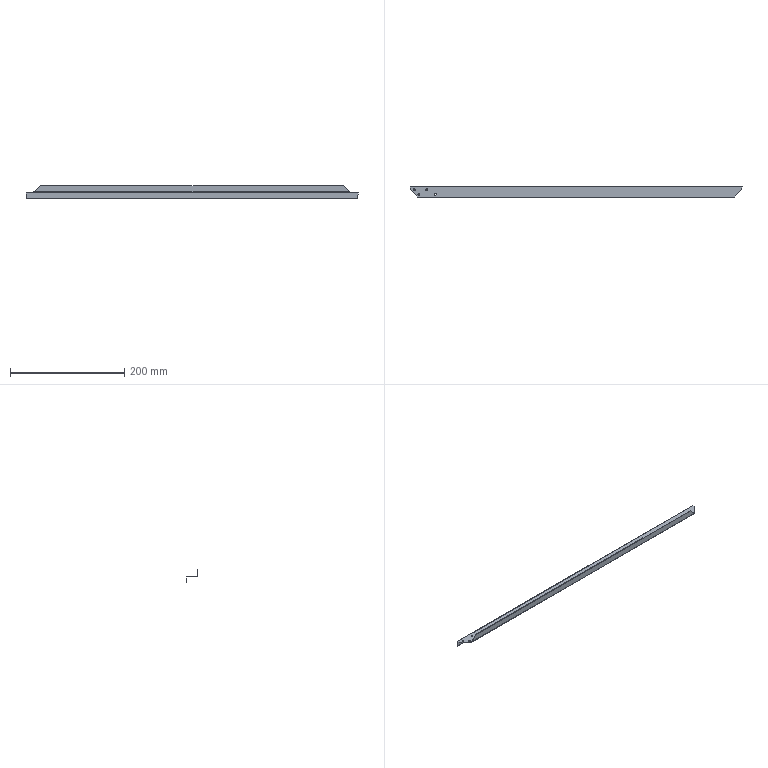Part | SolidWorks | features BaseBody 1 | 1 solid | 28 faces | box 580 x 20.861 x 22.562 mm | volume 11752 mm3 | plane 14 | cylinder 12 | spline 2 | commonest cylinder face diameters 3.2 x8 2 x2 3 x2
STEP:
#1=CARTESIAN_POINT('',(-272.991,-3.763,-0.5));
#2=VERTEX_POINT('',#1);
#3=CARTESIAN_POINT('',(-276.191,-3.763,-0.5));
#4=VERTEX_POINT('',#3);
#5=CARTESIAN_POINT('',(-274.591,-3.763,-0.5));
#6=DIRECTION('',(0.,0.,-1.));
#7=DIRECTION('',(1.,0.,0.));
#8=AXIS2_PLACEMENT_3D('',#5,#6,#7);
#9=CIRCLE('',#8,1.6);
#10=EDGE_CURVE('',#2,#4,#9,.T.);
#11=ORIENTED_EDGE('',*,*,#10,.T.);
#12=CARTESIAN_POINT('',(-276.191,-3.763,0.));
#13=VERTEX_POINT('',#12);
#14=CARTESIAN_POINT('',(-276.191,-3.763,-0.5));
#15=DIRECTION('',(0.,0.,1.));
#16=VECTOR('',#15,1000.);
#17=LINE('',#14,#16);
#18=EDGE_CURVE('',#4,#13,#17,.T.);
#19=ORIENTED_EDGE('',*,*,#18,.T.);
#20=CARTESIAN_POINT('',(-272.991,-3.763,0.));
#21=VERTEX_POINT('',#20);
#22=CARTESIAN_POINT('',(-274.591,-3.763,0.));
#23=DIRECTION('',(0.,0.,1.));
#24=DIRECTION('',(1.,0.,0.));
#25=AXIS2_PLACEMENT_3D('',#22,#23,#24);
#26=CIRCLE('',#25,1.6);
#27=EDGE_CURVE('',#13,#21,#26,.T.);
#28=ORIENTED_EDGE('',*,*,#27,.T.);
#29=CARTESIAN_POINT('',(-272.991,-3.763,-0.5));
#30=DIRECTION('',(0.,0.,1.));
#31=VECTOR('',#30,1000.);
#32=LINE('',#29,#31);
#33=EDGE_CURVE('',#2,#21,#32,.T.);
#34=ORIENTED_EDGE('',*,*,#33,.F.);
#35=EDGE_LOOP('',(#11,#19,#28,#34));
#36=FACE_OUTER_BOUND('',#35,.T.);
#37=CARTESIAN_POINT('',(-274.591,-3.763,-0.5));
#38=DIRECTION('',(0.,0.,1.));
#39=DIRECTION('',(1.,0.,0.));
#40=AXIS2_PLACEMENT_3D('',#37,#38,#39);
#41=CYLINDRICAL_SURFACE('',#40,1.6);
#42=ADVANCED_FACE('',(#36),#41,.F.);
#43=CARTESIAN_POINT('',(-284.191,4.237,-0.5));
#44=VERTEX_POINT('',#43);
#45=CARTESIAN_POINT('',(-280.991,4.237,-0.5));
#46=VERTEX_POINT('',#45);
#47=CARTESIAN_POINT('',(-282.591,4.237,-0.5));
#48=DIRECTION('',(0.,0.,1.));
#49=DIRECTION('',(1.,0.,0.));
#50=AXIS2_PLACEMENT_3D('',#47,#48,#49);
#51=CIRCLE('',#50,1.6);
#52=EDGE_CURVE('',#44,#46,#51,.T.);
#53=ORIENTED_EDGE('',*,*,#52,.F.);
#54=CARTESIAN_POINT('',(-284.191,4.237,0.));
#55=VERTEX_POINT('',#54);
#56=CARTESIAN_POINT('',(-284.191,4.237,-0.5));
#57=DIRECTION('',(0.,0.,1.));
#58=VECTOR('',#57,1000.);
#59=LINE('',#56,#58);
#60=EDGE_CURVE('',#44,#55,#59,.T.);
#61=ORIENTED_EDGE('',*,*,#60,.T.);
#62=CARTESIAN_POINT('',(-280.991,4.237,0.));
#63=VERTEX_POINT('',#62);
#64=CARTESIAN_POINT('',(-282.591,4.237,0.));
#65=DIRECTION('',(0.,0.,1.));
#66=DIRECTION('',(1.,0.,0.));
#67=AXIS2_PLACEMENT_3D('',#64,#65,#66);
#68=CIRCLE('',#67,1.6);
#69=EDGE_CURVE('',#55,#63,#68,.T.);
#70=ORIENTED_EDGE('',*,*,#69,.T.);
#71=CARTESIAN_POINT('',(-280.991,4.237,-0.5));
#72=DIRECTION('',(0.,0.,1.));
#73=VECTOR('',#72,1000.);
#74=LINE('',#71,#73);
#75=EDGE_CURVE('',#46,#63,#74,.T.);
#76=ORIENTED_EDGE('',*,*,#75,.F.);
#77=EDGE_LOOP('',(#53,#61,#70,#76));
#78=FACE_OUTER_BOUND('',#77,.T.);
#79=CARTESIAN_POINT('',(-282.591,4.237,-0.5));
#80=DIRECTION('',(0.,0.,1.));
#81=DIRECTION('',(1.,0.,0.));
#82=AXIS2_PLACEMENT_3D('',#79,#80,#81);
#83=CYLINDRICAL_SURFACE('',#82,1.6);
#84=ADVANCED_FACE('',(#78),#83,.F.);
#85=CARTESIAN_POINT('',(-262.191,4.237,-0.5));
#86=VERTEX_POINT('',#85);
#87=CARTESIAN_POINT('',(-258.991,4.237,-0.5));
#88=VERTEX_POINT('',#87);
#89=CARTESIAN_POINT('',(-260.591,4.237,-0.5));
#90=DIRECTION('',(0.,0.,1.));
#91=DIRECTION('',(1.,0.,0.));
#92=AXIS2_PLACEMENT_3D('',#89,#90,#91);
#93=CIRCLE('',#92,1.6);
#94=EDGE_CURVE('',#86,#88,#93,.T.);
#95=ORIENTED_EDGE('',*,*,#94,.F.);
#96=CARTESIAN_POINT('',(-262.191,4.237,0.));
#97=VERTEX_POINT('',#96);
#98=CARTESIAN_POINT('',(-262.191,4.237,-0.5));
#99=DIRECTION('',(0.,0.,1.));
#100=VECTOR('',#99,1000.);
#101=LINE('',#98,#100);
#102=EDGE_CURVE('',#86,#97,#101,.T.);
#103=ORIENTED_EDGE('',*,*,#102,.T.);
#104=CARTESIAN_POINT('',(-258.991,4.237,0.));
#105=VERTEX_POINT('',#104);
#106=CARTESIAN_POINT('',(-260.591,4.237,0.));
#107=DIRECTION('',(0.,0.,1.));
#108=DIRECTION('',(1.,0.,0.));
#109=AXIS2_PLACEMENT_3D('',#106,#107,#108);
#110=CIRCLE('',#109,1.6);
#111=EDGE_CURVE('',#97,#105,#110,.T.);
#112=ORIENTED_EDGE('',*,*,#111,.T.);
#113=CARTESIAN_POINT('',(-258.991,4.237,-0.5));
#114=DIRECTION('',(0.,0.,1.));
#115=VECTOR('',#114,1000.);
#116=LINE('',#113,#115);
#117=EDGE_CURVE('',#88,#105,#116,.T.);
#118=ORIENTED_EDGE('',*,*,#117,.F.);
#119=EDGE_LOOP('',(#95,#103,#112,#118));
#120=FACE_OUTER_BOUND('',#119,.T.);
#121=CARTESIAN_POINT('',(-260.591,4.237,-0.5));
#122=DIRECTION('',(0.,0.,1.));
#123=DIRECTION('',(1.,0.,0.));
#124=AXIS2_PLACEMENT_3D('',#121,#122,#123);
#125=CYLINDRICAL_SURFACE('',#124,1.6);
#126=ADVANCED_FACE('',(#120),#125,.F.);
#127=CARTESIAN_POINT('',(-247.581,-3.763,-0.5));
#128=VERTEX_POINT('',#127);
#129=CARTESIAN_POINT('',(-244.381,-3.763,-0.5));
#130=VERTEX_POINT('',#129);
#131=CARTESIAN_POINT('',(-245.981,-3.763,-0.5));
#132=DIRECTION('',(0.,0.,1.));
#133=DIRECTION('',(1.,0.,0.));
#134=AXIS2_PLACEMENT_3D('',#131,#132,#133);
#135=CIRCLE('',#134,1.6);
#136=EDGE_CURVE('',#128,#130,#135,.T.);
#137=ORIENTED_EDGE('',*,*,#136,.F.);
#138=CARTESIAN_POINT('',(-247.581,-3.763,0.));
#139=VERTEX_POINT('',#138);
#140=CARTESIAN_POINT('',(-247.581,-3.763,-0.5));
#141=DIRECTION('',(0.,0.,1.));
#142=VECTOR('',#141,1000.);
#143=LINE('',#140,#142);
#144=EDGE_CURVE('',#128,#139,#143,.T.);
#145=ORIENTED_EDGE('',*,*,#144,.T.);
#146=CARTESIAN_POINT('',(-244.381,-3.763,0.));
#147=VERTEX_POINT('',#146);
#148=CARTESIAN_POINT('',(-245.981,-3.763,0.));
#149=DIRECTION('',(0.,0.,1.));
#150=DIRECTION('',(1.,0.,0.));
#151=AXIS2_PLACEMENT_3D('',#148,#149,#150);
#152=CIRCLE('',#151,1.6);
#153=EDGE_CURVE('',#139,#147,#152,.T.);
#154=ORIENTED_EDGE('',*,*,#153,.T.);
#155=CARTESIAN_POINT('',(-244.381,-3.763,-0.5));
#156=DIRECTION('',(0.,0.,1.));
#157=VECTOR('',#156,1000.);
#158=LINE('',#155,#157);
#159=EDGE_CURVE('',#130,#147,#158,.T.);
#160=ORIENTED_EDGE('',*,*,#159,.F.);
#161=EDGE_LOOP('',(#137,#145,#154,#160));
#162=FACE_OUTER_BOUND('',#161,.T.);
#163=CARTESIAN_POINT('',(-245.981,-3.763,-0.5));
#164=DIRECTION('',(0.,0.,1.));
#165=DIRECTION('',(1.,0.,0.));
#166=AXIS2_PLACEMENT_3D('',#163,#164,#165);
#167=CYLINDRICAL_SURFACE('',#166,1.6);
#168=ADVANCED_FACE('',(#162),#167,.F.);
#169=ORIENTED_EDGE('',*,*,#18,.F.);
#170=CARTESIAN_POINT('',(-274.591,-3.763,-0.5));
#171=DIRECTION('',(0.,0.,-1.));
#172=DIRECTION('',(1.,0.,0.));
#173=AXIS2_PLACEMENT_3D('',#170,#171,#172);
#174=CIRCLE('',#173,1.6);
#175=EDGE_CURVE('',#4,#2,#174,.T.);
#176=ORIENTED_EDGE('',*,*,#175,.T.);
#177=ORIENTED_EDGE('',*,*,#33,.T.);
#178=CARTESIAN_POINT('',(-274.591,-3.763,0.));
#179=DIRECTION('',(0.,0.,1.));
#180=DIRECTION('',(1.,0.,0.));
#181=AXIS2_PLACEMENT_3D('',#178,#179,#180);
#182=CIRCLE('',#181,1.6);
#183=EDGE_CURVE('',#21,#13,#182,.T.);
#184=ORIENTED_EDGE('',*,*,#183,.T.);
#185=EDGE_LOOP('',(#169,#176,#177,#184));
#186=FACE_OUTER_BOUND('',#185,.T.);
#187=CARTESIAN_POINT('',(-274.591,-3.763,-0.5));
#188=DIRECTION('',(0.,0.,1.));
#189=DIRECTION('',(1.,0.,0.));
#190=AXIS2_PLACEMENT_3D('',#187,#188,#189);
#191=CYLINDRICAL_SURFACE('',#190,1.6);
#192=ADVANCED_FACE('',(#186),#191,.F.);
#193=CARTESIAN_POINT('',(-282.591,4.237,0.));
#194=DIRECTION('',(0.,0.,1.));
#195=DIRECTION('',(1.,0.,0.));
#196=AXIS2_PLACEMENT_3D('',#193,#194,#195);
#197=CIRCLE('',#196,1.6);
#198=EDGE_CURVE('',#63,#55,#197,.T.);
#199=ORIENTED_EDGE('',*,*,#198,.F.);
#200=ORIENTED_EDGE('',*,*,#69,.F.);
#201=EDGE_LOOP('',(#199,#200));
#202=FACE_BOUND('',#201,.T.);
#203=CARTESIAN_POINT('',(-260.591,4.237,0.));
#204=DIRECTION('',(0.,0.,1.));
#205=DIRECTION('',(1.,0.,0.));
#206=AXIS2_PLACEMENT_3D('',#203,#204,#205);
#207=CIRCLE('',#206,1.6);
#208=EDGE_CURVE('',#105,#97,#207,.T.);
#209=ORIENTED_EDGE('',*,*,#208,.F.);
#210=ORIENTED_EDGE('',*,*,#111,.F.);
#211=EDGE_LOOP('',(#209,#210));
#212=FACE_BOUND('',#211,.T.);
#213=CARTESIAN_POINT('',(-245.981,-3.763,0.));
#214=DIRECTION('',(0.,0.,1.));
#215=DIRECTION('',(1.,0.,0.));
#216=AXIS2_PLACEMENT_3D('',#213,#214,#215);
#217=CIRCLE('',#216,1.6);
#218=EDGE_CURVE('',#147,#139,#217,.T.);
#219=ORIENTED_EDGE('',*,*,#218,.F.);
#220=ORIENTED_EDGE('',*,*,#153,.F.);
#221=EDGE_LOOP('',(#219,#220));
#222=FACE_BOUND('',#221,.T.);
#223=ORIENTED_EDGE('',*,*,#183,.F.);
#224=ORIENTED_EDGE('',*,*,#27,.F.);
#225=EDGE_LOOP('',(#223,#224));
#226=FACE_BOUND('',#225,.T.);
#227=CARTESIAN_POINT('',(276.986,-8.364,0.));
#228=VERTEX_POINT('',#227);
#229=CARTESIAN_POINT('',(-276.986,-8.364,0.));
#230=VERTEX_POINT('',#229);
#231=CARTESIAN_POINT('',(0.,-8.364,0.));
#232=DIRECTION('',(-1.,0.,0.));
#233=VECTOR('',#232,1000.);
#234=LINE('',#231,#233);
#235=EDGE_CURVE('',#228,#230,#234,.T.);
#236=ORIENTED_EDGE('',*,*,#235,.F.);
#237=CARTESIAN_POINT('',(290.,4.65,0.));
#238=VERTEX_POINT('',#237);
#239=CARTESIAN_POINT('',(276.986,-8.364,0.));
#240=DIRECTION('',(-0.7071,-0.7071,0.));
#241=VECTOR('',#240,1000.);
#242=LINE('',#239,#241);
#243=EDGE_CURVE('',#238,#228,#242,.T.);
#244=ORIENTED_EDGE('',*,*,#243,.F.);
#245=CARTESIAN_POINT('',(290.,9.35,0.));
#246=VERTEX_POINT('',#245);
#247=CARTESIAN_POINT('',(290.,0.4931,0.));
#248=DIRECTION('',(0.,-1.,0.));
#249=VECTOR('',#248,1000.);
#250=LINE('',#247,#249);
#251=EDGE_CURVE('',#246,#238,#250,.T.);
#252=ORIENTED_EDGE('',*,*,#251,.F.);
#253=CARTESIAN_POINT('',(-290.,9.35,0.));
#254=VERTEX_POINT('',#253);
#255=CARTESIAN_POINT('',(0.,9.35,0.));
#256=DIRECTION('',(1.,0.,0.));
#257=VECTOR('',#256,1000.);
#258=LINE('',#255,#257);
#259=EDGE_CURVE('',#254,#246,#258,.T.);
#260=ORIENTED_EDGE('',*,*,#259,.F.);
#261=CARTESIAN_POINT('',(-290.,4.65,0.));
#262=VERTEX_POINT('',#261);
#263=CARTESIAN_POINT('',(-290.,0.4931,0.));
#264=DIRECTION('',(0.,1.,0.));
#265=VECTOR('',#264,1000.);
#266=LINE('',#263,#265);
#267=EDGE_CURVE('',#262,#254,#266,.T.);
#268=ORIENTED_EDGE('',*,*,#267,.F.);
#269=CARTESIAN_POINT('',(-290.,4.65,0.));
#270=DIRECTION('',(-0.7071,0.7071,0.));
#271=VECTOR('',#270,1000.);
#272=LINE('',#269,#271);
#273=EDGE_CURVE('',#230,#262,#272,.T.);
#274=ORIENTED_EDGE('',*,*,#273,.F.);
#275=EDGE_LOOP('',(#236,#244,#252,#260,#268,#274));
#276=FACE_OUTER_BOUND('',#275,.T.);
#277=CARTESIAN_POINT('',(290.,-8.364,0.));
#278=DIRECTION('',(0.,0.,-1.));
#279=DIRECTION('',(-1.,0.,0.));
#280=AXIS2_PLACEMENT_3D('',#277,#278,#279);
#281=PLANE('',#280);
#282=ADVANCED_FACE('',(#202,#212,#222,#226,#276),#281,.F.);
#283=CARTESIAN_POINT('',(-282.591,4.237,-0.5));
#284=DIRECTION('',(0.,0.,1.));
#285=DIRECTION('',(1.,0.,0.));
#286=AXIS2_PLACEMENT_3D('',#283,#284,#285);
#287=CIRCLE('',#286,1.6);
#288=EDGE_CURVE('',#46,#44,#287,.T.);
#289=ORIENTED_EDGE('',*,*,#288,.T.);
#290=ORIENTED_EDGE('',*,*,#52,.T.);
#291=EDGE_LOOP('',(#289,#290));
#292=FACE_BOUND('',#291,.T.);
#293=CARTESIAN_POINT('',(-260.591,4.237,-0.5));
#294=DIRECTION('',(0.,0.,1.));
#295=DIRECTION('',(1.,0.,0.));
#296=AXIS2_PLACEMENT_3D('',#293,#294,#295);
#297=CIRCLE('',#296,1.6);
#298=EDGE_CURVE('',#88,#86,#297,.T.);
#299=ORIENTED_EDGE('',*,*,#298,.T.);
#300=ORIENTED_EDGE('',*,*,#94,.T.);
#301=EDGE_LOOP('',(#299,#300));
#302=FACE_BOUND('',#301,.T.);
#303=CARTESIAN_POINT('',(-245.981,-3.763,-0.5));
#304=DIRECTION('',(0.,0.,1.));
#305=DIRECTION('',(1.,0.,0.));
#306=AXIS2_PLACEMENT_3D('',#303,#304,#305);
#307=CIRCLE('',#306,1.6);
#308=EDGE_CURVE('',#130,#128,#307,.T.);
#309=ORIENTED_EDGE('',*,*,#308,.T.);
#310=ORIENTED_EDGE('',*,*,#136,.T.);
#311=EDGE_LOOP('',(#309,#310));
#312=FACE_BOUND('',#311,.T.);
#313=ORIENTED_EDGE('',*,*,#10,.F.);
#314=ORIENTED_EDGE('',*,*,#175,.F.);
#315=EDGE_LOOP('',(#313,#314));
#316=FACE_BOUND('',#315,.T.);
#317=CARTESIAN_POINT('',(290.,9.35,-0.5));
#318=VERTEX_POINT('',#317);
#319=CARTESIAN_POINT('',(290.,4.65,-0.5));
#320=VERTEX_POINT('',#319);
#321=CARTESIAN_POINT('',(290.,0.4931,-0.5));
#322=DIRECTION('',(0.,-1.,0.));
#323=VECTOR('',#322,1000.);
#324=LINE('',#321,#323);
#325=EDGE_CURVE('',#318,#320,#324,.T.);
#326=ORIENTED_EDGE('',*,*,#325,.T.);
#327=CARTESIAN_POINT('',(276.986,-8.364,-0.5));
#328=VERTEX_POINT('',#327);
#329=CARTESIAN_POINT('',(290.,4.65,-0.5));
#330=DIRECTION('',(-0.7071,-0.7071,0.));
#331=VECTOR('',#330,1000.);
#332=LINE('',#329,#331);
#333=EDGE_CURVE('',#320,#328,#332,.T.);
#334=ORIENTED_EDGE('',*,*,#333,.T.);
#335=CARTESIAN_POINT('',(-276.986,-8.364,-0.5));
#336=VERTEX_POINT('',#335);
#337=CARTESIAN_POINT('',(0.,-8.364,-0.5));
#338=DIRECTION('',(-1.,0.,0.));
#339=VECTOR('',#338,1000.);
#340=LINE('',#337,#339);
#341=EDGE_CURVE('',#328,#336,#340,.T.);
#342=ORIENTED_EDGE('',*,*,#341,.T.);
#343=CARTESIAN_POINT('',(-290.,4.65,-0.5));
#344=VERTEX_POINT('',#343);
#345=CARTESIAN_POINT('',(-276.986,-8.364,-0.5));
#346=DIRECTION('',(-0.7071,0.7071,0.));
#347=VECTOR('',#346,1000.);
#348=LINE('',#345,#347);
#349=EDGE_CURVE('',#336,#344,#348,.T.);
#350=ORIENTED_EDGE('',*,*,#349,.T.);
#351=CARTESIAN_POINT('',(-290.,9.35,-0.5));
#352=VERTEX_POINT('',#351);
#353=CARTESIAN_POINT('',(-290.,0.4931,-0.5));
#354=DIRECTION('',(0.,1.,0.));
#355=VECTOR('',#354,1000.);
#356=LINE('',#353,#355);
#357=EDGE_CURVE('',#344,#352,#356,.T.);
#358=ORIENTED_EDGE('',*,*,#357,.T.);
#359=CARTESIAN_POINT('',(0.,9.35,-0.5));
#360=DIRECTION('',(1.,0.,0.));
#361=VECTOR('',#360,1000.);
#362=LINE('',#359,#361);
#363=EDGE_CURVE('',#352,#318,#362,.T.);
#364=ORIENTED_EDGE('',*,*,#363,.T.);
#365=EDGE_LOOP('',(#326,#334,#342,#350,#358,#364));
#366=FACE_OUTER_BOUND('',#365,.T.);
#367=CARTESIAN_POINT('',(290.,-8.364,-0.5));
#368=DIRECTION('',(0.,0.,-1.));
#369=DIRECTION('',(-1.,0.,0.));
#370=AXIS2_PLACEMENT_3D('',#367,#368,#369);
#371=PLANE('',#370);
#372=ADVANCED_FACE('',(#292,#302,#312,#316,#366),#371,.T.);
#373=ORIENTED_EDGE('',*,*,#60,.F.);
#374=ORIENTED_EDGE('',*,*,#288,.F.);
#375=ORIENTED_EDGE('',*,*,#75,.T.);
#376=ORIENTED_EDGE('',*,*,#198,.T.);
#377=EDGE_LOOP('',(#373,#374,#375,#376));
#378=FACE_OUTER_BOUND('',#377,.T.);
#379=CARTESIAN_POINT('',(-282.591,4.237,-0.5));
#380=DIRECTION('',(0.,0.,1.));
#381=DIRECTION('',(1.,0.,0.));
#382=AXIS2_PLACEMENT_3D('',#379,#380,#381);
#383=CYLINDRICAL_SURFACE('',#382,1.6);
#384=ADVANCED_FACE('',(#378),#383,.F.);
#385=ORIENTED_EDGE('',*,*,#102,.F.);
#386=ORIENTED_EDGE('',*,*,#298,.F.);
#387=ORIENTED_EDGE('',*,*,#117,.T.);
#388=ORIENTED_EDGE('',*,*,#208,.T.);
#389=EDGE_LOOP('',(#385,#386,#387,#388));
#390=FACE_OUTER_BOUND('',#389,.T.);
#391=CARTESIAN_POINT('',(-260.591,4.237,-0.5));
#392=DIRECTION('',(0.,0.,1.));
#393=DIRECTION('',(1.,0.,0.));
#394=AXIS2_PLACEMENT_3D('',#391,#392,#393);
#395=CYLINDRICAL_SURFACE('',#394,1.6);
#396=ADVANCED_FACE('',(#390),#395,.F.);
#397=ORIENTED_EDGE('',*,*,#144,.F.);
#398=ORIENTED_EDGE('',*,*,#308,.F.);
#399=ORIENTED_EDGE('',*,*,#159,.T.);
#400=ORIENTED_EDGE('',*,*,#218,.T.);
#401=EDGE_LOOP('',(#397,#398,#399,#400));
#402=FACE_OUTER_BOUND('',#401,.T.);
#403=CARTESIAN_POINT('',(-245.981,-3.763,-0.5));
#404=DIRECTION('',(0.,0.,1.));
#405=DIRECTION('',(1.,0.,0.));
#406=AXIS2_PLACEMENT_3D('',#403,#404,#405);
#407=CYLINDRICAL_SURFACE('',#406,1.6);
#408=ADVANCED_FACE('',(#402),#407,.F.);
#409=CARTESIAN_POINT('',(-290.,4.65,-0.25));
#410=DIRECTION('',(0.,0.,-1.));
#411=VECTOR('',#410,1000.);
#412=LINE('',#409,#411);
#413=EDGE_CURVE('',#262,#344,#412,.T.);
#414=ORIENTED_EDGE('',*,*,#413,.T.);
#415=ORIENTED_EDGE('',*,*,#349,.F.);
#416=CARTESIAN_POINT('',(-276.986,-8.364,-0.25));
#417=DIRECTION('',(0.,0.,-1.));
#418=VECTOR('',#417,1000.);
#419=LINE('',#416,#418);
#420=EDGE_CURVE('',#230,#336,#419,.T.);
#421=ORIENTED_EDGE('',*,*,#420,.F.);
#422=ORIENTED_EDGE('',*,*,#273,.T.);
#423=EDGE_LOOP('',(#414,#415,#421,#422));
#424=FACE_OUTER_BOUND('',#423,.T.);
#425=CARTESIAN_POINT('',(-290.,4.65,-0.5));
#426=DIRECTION('',(-0.7071,-0.7071,0.));
#427=DIRECTION('',(0.7071,-0.7071,0.));
#428=AXIS2_PLACEMENT_3D('',#425,#426,#427);
#429=PLANE('',#428);
#430=ADVANCED_FACE('',(#424),#429,.T.);
#431=CARTESIAN_POINT('',(-275.04,-9.364,0.986));
#432=VERTEX_POINT('',#431);
#433=CARTESIAN_POINT('',(275.04,-9.364,0.986));
#434=VERTEX_POINT('',#433);
#435=CARTESIAN_POINT('',(0.,-9.364,0.986));
#436=DIRECTION('',(1.,0.,0.));
#437=VECTOR('',#436,1000.);
#438=LINE('',#435,#437);
#439=EDGE_CURVE('',#432,#434,#438,.T.);
#440=ORIENTED_EDGE('',*,*,#439,.T.);
#441=CARTESIAN_POINT('',(275.04,-9.364,0.986));
#442=CARTESIAN_POINT('',(275.204,-9.362,0.8552));
#443=CARTESIAN_POINT('',(275.364,-9.335,0.7274));
#444=CARTESIAN_POINT('',(275.687,-9.233,0.4893));
#445=CARTESIAN_POINT('',(275.851,-9.158,0.3789));
#446=CARTESIAN_POINT('',(276.174,-8.974,0.1976));
#447=CARTESIAN_POINT('',(276.337,-8.864,0.1243));
#448=CARTESIAN_POINT('',(276.662,-8.623,0.02551));
#449=CARTESIAN_POINT('',(276.823,-8.495,0.000000001));
#450=CARTESIAN_POINT('',(276.986,-8.364,0.));
#451=B_SPLINE_CURVE_WITH_KNOTS('',3,(#441,#442,#443,#444,#445,#446,#447,#448,#449,#450),.UNSPECIFIED.,.F.,.F.,(4,2,2,2,4),(0.,0.0006197,0.001239,0.001859,0.002479),.UNSPECIFIED.);
#452=EDGE_CURVE('',#434,#228,#451,.T.);
#453=ORIENTED_EDGE('',*,*,#452,.T.);
#454=ORIENTED_EDGE('',*,*,#235,.T.);
#455=CARTESIAN_POINT('',(-276.986,-8.364,0.));
#456=CARTESIAN_POINT('',(-276.823,-8.495,0.000000002));
#457=CARTESIAN_POINT('',(-276.662,-8.623,0.02551));
#458=CARTESIAN_POINT('',(-276.339,-8.862,0.1235));
#459=CARTESIAN_POINT('',(-276.175,-8.974,0.1971));
#460=CARTESIAN_POINT('',(-275.852,-9.158,0.3783));
#461=CARTESIAN_POINT('',(-275.689,-9.233,0.4878));
#462=CARTESIAN_POINT('',(-275.364,-9.335,0.727));
#463=CARTESIAN_POINT('',(-275.204,-9.362,0.8552));
#464=CARTESIAN_POINT('',(-275.04,-9.364,0.986));
#465=B_SPLINE_CURVE_WITH_KNOTS('',3,(#455,#456,#457,#458,#459,#460,#461,#462,#463,#464),.UNSPECIFIED.,.F.,.F.,(4,2,2,2,4),(0.,0.0006197,0.001239,0.001859,0.002479),.UNSPECIFIED.);
#466=EDGE_CURVE('',#230,#432,#465,.T.);
#467=ORIENTED_EDGE('',*,*,#466,.T.);
#468=EDGE_LOOP('',(#440,#453,#454,#467));
#469=FACE_OUTER_BOUND('',#468,.T.);
#470=CARTESIAN_POINT('',(280.31,-8.364,1.));
#471=DIRECTION('',(-1.,0.,0.));
#472=DIRECTION('',(0.,0.,1.));
#473=AXIS2_PLACEMENT_3D('',#470,#471,#472);
#474=CYLINDRICAL_SURFACE('',#473,1.);
#475=ADVANCED_FACE('',(#469),#474,.F.);
#476=CARTESIAN_POINT('',(290.,4.65,-0.25));
#477=DIRECTION('',(0.,0.,1.));
#478=VECTOR('',#477,1000.);
#479=LINE('',#476,#478);
#480=EDGE_CURVE('',#320,#238,#479,.T.);
#481=ORIENTED_EDGE('',*,*,#480,.T.);
#482=ORIENTED_EDGE('',*,*,#243,.T.);
#483=CARTESIAN_POINT('',(276.986,-8.364,-0.25));
#484=DIRECTION('',(0.,0.,-1.));
#485=VECTOR('',#484,1000.);
#486=LINE('',#483,#485);
#487=EDGE_CURVE('',#228,#328,#486,.T.);
#488=ORIENTED_EDGE('',*,*,#487,.T.);
#489=ORIENTED_EDGE('',*,*,#333,.F.);
#490=EDGE_LOOP('',(#481,#482,#488,#489));
#491=FACE_OUTER_BOUND('',#490,.T.);
#492=CARTESIAN_POINT('',(276.986,-8.364,-0.5));
#493=DIRECTION('',(0.7071,-0.7071,0.));
#494=DIRECTION('',(0.7071,0.7071,0.));
#495=AXIS2_PLACEMENT_3D('',#492,#493,#494);
#496=PLANE('',#495);
#497=ADVANCED_FACE('',(#491),#496,.T.);
#498=ORIENTED_EDGE('',*,*,#251,.T.);
#499=ORIENTED_EDGE('',*,*,#480,.F.);
#500=ORIENTED_EDGE('',*,*,#325,.F.);
#501=CARTESIAN_POINT('',(290.,10.35,-1.5));
#502=VERTEX_POINT('',#501);
#503=CARTESIAN_POINT('',(290.,9.35,-1.5));
#504=DIRECTION('',(1.,0.,0.));
#505=DIRECTION('',(0.,1.,0.));
#506=AXIS2_PLACEMENT_3D('',#503,#504,#505);
#507=CIRCLE('',#506,1.);
#508=EDGE_CURVE('',#502,#318,#507,.T.);
#509=ORIENTED_EDGE('',*,*,#508,.F.);
#510=CARTESIAN_POINT('',(290.,10.35,-11.037));
#511=VERTEX_POINT('',#510);
#512=CARTESIAN_POINT('',(290.,10.35,-6.268));
#513=DIRECTION('',(0.,0.,1.));
#514=VECTOR('',#513,1000.);
#515=LINE('',#512,#514);
#516=EDGE_CURVE('',#511,#502,#515,.T.);
#517=ORIENTED_EDGE('',*,*,#516,.F.);
#518=CARTESIAN_POINT('',(290.,10.85,-11.037));
#519=VERTEX_POINT('',#518);
#520=CARTESIAN_POINT('',(290.,10.6,-11.037));
#521=DIRECTION('',(0.,1.,0.));
#522=VECTOR('',#521,1000.);
#523=LINE('',#520,#522);
#524=EDGE_CURVE('',#511,#519,#523,.T.);
#525=ORIENTED_EDGE('',*,*,#524,.T.);
#526=CARTESIAN_POINT('',(290.,10.85,-1.5));
#527=VERTEX_POINT('',#526);
#528=CARTESIAN_POINT('',(290.,10.85,-6.268));
#529=DIRECTION('',(0.,0.,1.));
#530=VECTOR('',#529,1000.);
#531=LINE('',#528,#530);
#532=EDGE_CURVE('',#519,#527,#531,.T.);
#533=ORIENTED_EDGE('',*,*,#532,.T.);
#534=CARTESIAN_POINT('',(290.,9.35,-1.5));
#535=DIRECTION('',(1.,0.,0.));
#536=DIRECTION('',(0.,1.,0.));
#537=AXIS2_PLACEMENT_3D('',#534,#535,#536);
#538=CIRCLE('',#537,1.5);
#539=EDGE_CURVE('',#527,#246,#538,.T.);
#540=ORIENTED_EDGE('',*,*,#539,.T.);
#541=EDGE_LOOP('',(#498,#499,#500,#509,#517,#525,#533,#540));
#542=FACE_OUTER_BOUND('',#541,.T.);
#543=CARTESIAN_POINT('',(290.,4.65,-0.5));
#544=DIRECTION('',(1.,0.,0.));
#545=DIRECTION('',(0.,1.,0.));
#546=AXIS2_PLACEMENT_3D('',#543,#544,#545);
#547=PLANE('',#546);
#548=ADVANCED_FACE('',(#542),#547,.T.);
#549=CARTESIAN_POINT('',(-290.,10.85,-1.5));
#550=VERTEX_POINT('',#549);
#551=CARTESIAN_POINT('',(0.,10.85,-1.5));
#552=DIRECTION('',(1.,0.,0.));
#553=VECTOR('',#552,1000.);
#554=LINE('',#551,#553);
#555=EDGE_CURVE('',#550,#527,#554,.T.);
#556=ORIENTED_EDGE('',*,*,#555,.F.);
#557=CARTESIAN_POINT('',(-290.,9.35,-1.5));
#558=DIRECTION('',(-1.,0.,0.));
#559=DIRECTION('',(0.,1.,0.));
#560=AXIS2_PLACEMENT_3D('',#557,#558,#559);
#561=CIRCLE('',#560,1.5);
#562=EDGE_CURVE('',#254,#550,#561,.T.);
#563=ORIENTED_EDGE('',*,*,#562,.F.);
#564=ORIENTED_EDGE('',*,*,#259,.T.);
#565=ORIENTED_EDGE('',*,*,#539,.F.);
#566=EDGE_LOOP('',(#556,#563,#564,#565));
#567=FACE_OUTER_BOUND('',#566,.T.);
#568=CARTESIAN_POINT('',(-290.,9.35,-1.5));
#569=DIRECTION('',(1.,0.,0.));
#570=DIRECTION('',(0.,1.,0.));
#571=AXIS2_PLACEMENT_3D('',#568,#569,#570);
#572=CYLINDRICAL_SURFACE('',#571,1.5);
#573=ADVANCED_FACE('',(#567),#572,.T.);
#574=ORIENTED_EDGE('',*,*,#357,.F.);
#575=ORIENTED_EDGE('',*,*,#413,.F.);
#576=ORIENTED_EDGE('',*,*,#267,.T.);
#577=ORIENTED_EDGE('',*,*,#562,.T.);
#578=CARTESIAN_POINT('',(-290.,10.85,-11.037));
#579=VERTEX_POINT('',#578);
#580=CARTESIAN_POINT('',(-290.,10.85,-6.268));
#581=DIRECTION('',(0.,0.,-1.));
#582=VECTOR('',#581,1000.);
#583=LINE('',#580,#582);
#584=EDGE_CURVE('',#550,#579,#583,.T.);
#585=ORIENTED_EDGE('',*,*,#584,.T.);
#586=CARTESIAN_POINT('',(-290.,10.35,-11.037));
#587=VERTEX_POINT('',#586);
#588=CARTESIAN_POINT('',(-290.,10.6,-11.037));
#589=DIRECTION('',(0.,-1.,0.));
#590=VECTOR('',#589,1000.);
#591=LINE('',#588,#590);
#592=EDGE_CURVE('',#579,#587,#591,.T.);
#593=ORIENTED_EDGE('',*,*,#592,.T.);
#594=CARTESIAN_POINT('',(-290.,10.35,-1.5));
#595=VERTEX_POINT('',#594);
#596=CARTESIAN_POINT('',(-290.,10.35,-6.268));
#597=DIRECTION('',(0.,0.,-1.));
#598=VECTOR('',#597,1000.);
#599=LINE('',#596,#598);
#600=EDGE_CURVE('',#595,#587,#599,.T.);
#601=ORIENTED_EDGE('',*,*,#600,.F.);
#602=CARTESIAN_POINT('',(-290.,9.35,-1.5));
#603=DIRECTION('',(-1.,0.,0.));
#604=DIRECTION('',(0.,1.,0.));
#605=AXIS2_PLACEMENT_3D('',#602,#603,#604);
#606=CIRCLE('',#605,1.);
#607=EDGE_CURVE('',#352,#595,#606,.T.);
#608=ORIENTED_EDGE('',*,*,#607,.F.);
#609=EDGE_LOOP('',(#574,#575,#576,#577,#585,#593,#601,#608));
#610=FACE_OUTER_BOUND('',#609,.T.);
#611=CARTESIAN_POINT('',(-290.,4.65,-0.5));
#612=DIRECTION('',(-1.,0.,0.));
#613=DIRECTION('',(0.,0.,1.));
#614=AXIS2_PLACEMENT_3D('',#611,#612,#613);
#615=PLANE('',#614);
#616=ADVANCED_FACE('',(#610),#615,.T.);
#617=ORIENTED_EDGE('',*,*,#607,.T.);
#618=CARTESIAN_POINT('',(0.,10.35,-1.5));
#619=DIRECTION('',(1.,0.,0.));
#620=VECTOR('',#619,1000.);
#621=LINE('',#618,#620);
#622=EDGE_CURVE('',#595,#502,#621,.T.);
#623=ORIENTED_EDGE('',*,*,#622,.T.);
#624=ORIENTED_EDGE('',*,*,#508,.T.);
#625=ORIENTED_EDGE('',*,*,#363,.F.);
#626=EDGE_LOOP('',(#617,#623,#624,#625));
#627=FACE_OUTER_BOUND('',#626,.T.);
#628=CARTESIAN_POINT('',(-290.,9.35,-1.5));
#629=DIRECTION('',(1.,0.,0.));
#630=DIRECTION('',(0.,1.,0.));
#631=AXIS2_PLACEMENT_3D('',#628,#629,#630);
#632=CYLINDRICAL_SURFACE('',#631,1.);
#633=ADVANCED_FACE('',(#627),#632,.F.);
#634=CARTESIAN_POINT('',(275.04,-9.864,0.9791));
#635=VERTEX_POINT('',#634);
#636=CARTESIAN_POINT('',(275.04,-9.864,0.9791));
#637=CARTESIAN_POINT('',(275.204,-9.861,0.7828));
#638=CARTESIAN_POINT('',(275.363,-9.82,0.592));
#639=CARTESIAN_POINT('',(275.607,-9.706,0.3227));
#640=CARTESIAN_POINT('',(275.689,-9.659,0.2363));
#641=CARTESIAN_POINT('',(275.85,-9.549,0.07602));
#642=CARTESIAN_POINT('',(275.931,-9.487,0.001505));
#643=CARTESIAN_POINT('',(276.093,-9.349,-0.1351));
#644=CARTESIAN_POINT('',(276.175,-9.272,-0.1974));
#645=CARTESIAN_POINT('',(276.337,-9.11,-0.3047));
#646=CARTESIAN_POINT('',(276.417,-9.025,-0.3501));
#647=CARTESIAN_POINT('',(276.659,-8.756,-0.4607));
#648=CARTESIAN_POINT('',(276.823,-8.56,-0.5));
#649=CARTESIAN_POINT('',(276.986,-8.364,-0.5));
#650=B_SPLINE_CURVE_WITH_KNOTS('',3,(#636,#637,#638,#639,#640,#641,#642,#643,#644,#645,#646,#647,#648,#649),.UNSPECIFIED.,.F.,.F.,(4,2,2,2,2,2,4),(0.,0.0007556,0.001133,0.001511,0.001889,0.002267,0.003022),.UNSPECIFIED.);
#651=EDGE_CURVE('',#635,#328,#650,.T.);
#652=ORIENTED_EDGE('',*,*,#651,.F.);
#653=CARTESIAN_POINT('',(-275.04,-9.864,0.9791));
#654=VERTEX_POINT('',#653);
#655=CARTESIAN_POINT('',(0.,-9.864,0.9791));
#656=DIRECTION('',(1.,0.,0.));
#657=VECTOR('',#656,1000.);
#658=LINE('',#655,#657);
#659=EDGE_CURVE('',#654,#635,#658,.T.);
#660=ORIENTED_EDGE('',*,*,#659,.F.);
#661=CARTESIAN_POINT('',(-276.986,-8.364,-0.5));
#662=CARTESIAN_POINT('',(-276.823,-8.56,-0.5));
#663=CARTESIAN_POINT('',(-276.663,-8.751,-0.4621));
#664=CARTESIAN_POINT('',(-276.419,-9.022,-0.3513));
#665=CARTESIAN_POINT('',(-276.337,-9.109,-0.3052));
#666=CARTESIAN_POINT('',(-276.176,-9.271,-0.1984));
#667=CARTESIAN_POINT('',(-276.096,-9.347,-0.1374));
#668=CARTESIAN_POINT('',(-275.934,-9.485,-0.001165));
#669=CARTESIAN_POINT('',(-275.852,-9.549,0.07475));
#670=CARTESIAN_POINT('',(-275.69,-9.658,0.2354));
#671=CARTESIAN_POINT('',(-275.609,-9.705,0.3204));
#672=CARTESIAN_POINT('',(-275.367,-9.819,0.5875));
#673=CARTESIAN_POINT('',(-275.204,-9.861,0.7828));
#674=CARTESIAN_POINT('',(-275.04,-9.864,0.9791));
#675=B_SPLINE_CURVE_WITH_KNOTS('',3,(#661,#662,#663,#664,#665,#666,#667,#668,#669,#670,#671,#672,#673,#674),.UNSPECIFIED.,.F.,.F.,(4,2,2,2,2,2,4),(0.,0.0007556,0.001133,0.001511,0.001889,0.002267,0.003022),.UNSPECIFIED.);
#676=EDGE_CURVE('',#336,#654,#675,.T.);
#677=ORIENTED_EDGE('',*,*,#676,.F.);
#678=ORIENTED_EDGE('',*,*,#341,.F.);
#679=EDGE_LOOP('',(#652,#660,#677,#678));
#680=FACE_OUTER_BOUND('',#679,.T.);
#681=CARTESIAN_POINT('',(280.31,-8.364,1.));
#682=DIRECTION('',(-1.,0.,0.));
#683=DIRECTION('',(0.,0.,1.));
#684=AXIS2_PLACEMENT_3D('',#681,#682,#683);
#685=CYLINDRICAL_SURFACE('',#684,1.5);
#686=ADVANCED_FACE('',(#680),#685,.T.);
#687=ORIENTED_EDGE('',*,*,#651,.T.);
#688=ORIENTED_EDGE('',*,*,#487,.F.);
#689=ORIENTED_EDGE('',*,*,#452,.F.);
#690=CARTESIAN_POINT('',(275.04,-9.614,0.9825));
#691=DIRECTION('',(0.,0.9999,0.01396));
#692=VECTOR('',#691,1000.);
#693=LINE('',#690,#692);
#694=EDGE_CURVE('',#635,#434,#693,.T.);
#695=ORIENTED_EDGE('',*,*,#694,.F.);
#696=EDGE_LOOP('',(#687,#688,#689,#695));
#697=FACE_OUTER_BOUND('',#696,.T.);
#698=CARTESIAN_POINT('',(276.986,-8.364,-0.505));
#699=CARTESIAN_POINT('',(276.824,-8.559,-0.505));
#700=CARTESIAN_POINT('',(276.662,-8.754,-0.4666));
#701=CARTESIAN_POINT('',(276.337,-9.116,-0.3184));
#702=CARTESIAN_POINT('',(276.175,-9.282,-0.2087));
#703=CARTESIAN_POINT('',(275.851,-9.56,0.06547));
#704=CARTESIAN_POINT('',(275.689,-9.672,0.2299));
#705=CARTESIAN_POINT('',(275.364,-9.825,0.5891));
#706=CARTESIAN_POINT('',(275.202,-9.866,0.7837));
#707=CARTESIAN_POINT('',(275.04,-9.869,0.979));
#708=CARTESIAN_POINT('',(276.986,-8.364,-0.5));
#709=CARTESIAN_POINT('',(276.824,-8.558,-0.5));
#710=CARTESIAN_POINT('',(276.662,-8.753,-0.4617));
#711=CARTESIAN_POINT('',(276.337,-9.113,-0.314));
#712=CARTESIAN_POINT('',(276.175,-9.279,-0.2047));
#713=CARTESIAN_POINT('',(275.851,-9.556,0.0686));
#714=CARTESIAN_POINT('',(275.689,-9.667,0.2325));
#715=CARTESIAN_POINT('',(275.364,-9.82,0.5905));
#716=CARTESIAN_POINT('',(275.202,-9.861,0.7845));
#717=CARTESIAN_POINT('',(275.04,-9.864,0.9791));
#718=CARTESIAN_POINT('',(276.986,-8.364,0.));
#719=CARTESIAN_POINT('',(276.824,-8.494,0.));
#720=CARTESIAN_POINT('',(276.662,-8.623,0.02556));
#721=CARTESIAN_POINT('',(276.337,-8.863,0.124));
#722=CARTESIAN_POINT('',(276.175,-8.974,0.1969));
#723=CARTESIAN_POINT('',(275.851,-9.158,0.3791));
#724=CARTESIAN_POINT('',(275.689,-9.233,0.4883));
#725=CARTESIAN_POINT('',(275.364,-9.335,0.727));
#726=CARTESIAN_POINT('',(275.202,-9.362,0.8563));
#727=CARTESIAN_POINT('',(275.04,-9.364,0.986));
#728=CARTESIAN_POINT('',(276.986,-8.364,0.005));
#729=CARTESIAN_POINT('',(276.824,-8.493,0.005));
#730=CARTESIAN_POINT('',(276.662,-8.622,0.03043));
#731=CARTESIAN_POINT('',(276.337,-8.861,0.1284));
#732=CARTESIAN_POINT('',(276.175,-8.971,0.2009));
#733=CARTESIAN_POINT('',(275.851,-9.154,0.3822));
#734=CARTESIAN_POINT('',(275.689,-9.228,0.4909));
#735=CARTESIAN_POINT('',(275.364,-9.33,0.7284));
#736=CARTESIAN_POINT('',(275.202,-9.357,0.857));
#737=CARTESIAN_POINT('',(275.04,-9.359,0.9861));
#738=B_SPLINE_SURFACE_WITH_KNOTS('',1,3,((#698,#699,#700,#701,#702,#703,#704,#705,#706,#707),(#708,#709,#710,#711,#712,#713,#714,#715,#716,#717),(#718,#719,#720,#721,#722,#723,#724,#725,#726,#727),(#728,#729,#730,#731,#732,#733,#734,#735,#736,#737)),.UNSPECIFIED.,.F.,.F.,.F.,(2,1,1,2),(4,2,2,2,4),(-0.0101,0.,1.,1.01),(0.,0.25,0.5,0.75,1.),.UNSPECIFIED.);
#739=ADVANCED_FACE('',(#697),#738,.T.);
#740=CARTESIAN_POINT('',(-264.5,-9.511,11.525));
#741=VERTEX_POINT('',#740);
#742=CARTESIAN_POINT('',(-275.04,-9.364,0.986));
#743=DIRECTION('',(-0.7071,0.009873,-0.707));
#744=VECTOR('',#743,1000.);
#745=LINE('',#742,#744);
#746=EDGE_CURVE('',#741,#432,#745,.T.);
#747=ORIENTED_EDGE('',*,*,#746,.F.);
#748=CARTESIAN_POINT('',(264.5,-9.511,11.525));
#749=VERTEX_POINT('',#748);
#750=CARTESIAN_POINT('',(0.,-9.511,11.525));
#751=DIRECTION('',(-1.,0.,0.));
#752=VECTOR('',#751,1000.);
#753=LINE('',#750,#752);
#754=EDGE_CURVE('',#749,#741,#753,.T.);
#755=ORIENTED_EDGE('',*,*,#754,.F.);
#756=CARTESIAN_POINT('',(264.5,-9.511,11.525));
#757=DIRECTION('',(-0.7071,-0.009873,0.707));
#758=VECTOR('',#757,1000.);
#759=LINE('',#756,#758);
#760=EDGE_CURVE('',#434,#749,#759,.T.);
#761=ORIENTED_EDGE('',*,*,#760,.F.);
#762=ORIENTED_EDGE('',*,*,#439,.F.);
#763=EDGE_LOOP('',(#747,#755,#761,#762));
#764=FACE_OUTER_BOUND('',#763,.T.);
#765=CARTESIAN_POINT('',(278.341,-9.511,11.525));
#766=DIRECTION('',(0.,-0.9999,-0.01396));
#767=DIRECTION('',(-1.,0.,0.));
#768=AXIS2_PLACEMENT_3D('',#765,#766,#767);
#769=PLANE('',#768);
#770=ADVANCED_FACE('',(#764),#769,.F.);
#771=ORIENTED_EDGE('',*,*,#420,.T.);
#772=ORIENTED_EDGE('',*,*,#676,.T.);
#773=CARTESIAN_POINT('',(-275.04,-9.614,0.9825));
#774=DIRECTION('',(0.,0.9999,0.01396));
#775=VECTOR('',#774,1000.);
#776=LINE('',#773,#775);
#777=EDGE_CURVE('',#654,#432,#776,.T.);
#778=ORIENTED_EDGE('',*,*,#777,.T.);
#779=ORIENTED_EDGE('',*,*,#466,.F.);
#780=EDGE_LOOP('',(#771,#772,#778,#779));
#781=FACE_OUTER_BOUND('',#780,.T.);
#782=CARTESIAN_POINT('',(-275.04,-9.869,0.979));
#783=CARTESIAN_POINT('',(-275.202,-9.866,0.7837));
#784=CARTESIAN_POINT('',(-275.364,-9.825,0.5891));
#785=CARTESIAN_POINT('',(-275.689,-9.672,0.2299));
#786=CARTESIAN_POINT('',(-275.851,-9.56,0.06547));
#787=CARTESIAN_POINT('',(-276.175,-9.282,-0.2087));
#788=CARTESIAN_POINT('',(-276.337,-9.116,-0.3184));
#789=CARTESIAN_POINT('',(-276.662,-8.754,-0.4666));
#790=CARTESIAN_POINT('',(-276.824,-8.559,-0.505));
#791=CARTESIAN_POINT('',(-276.986,-8.364,-0.505));
#792=CARTESIAN_POINT('',(-275.04,-9.864,0.9791));
#793=CARTESIAN_POINT('',(-275.202,-9.861,0.7845));
#794=CARTESIAN_POINT('',(-275.364,-9.82,0.5905));
#795=CARTESIAN_POINT('',(-275.689,-9.667,0.2325));
#796=CARTESIAN_POINT('',(-275.851,-9.556,0.0686));
#797=CARTESIAN_POINT('',(-276.175,-9.279,-0.2047));
#798=CARTESIAN_POINT('',(-276.337,-9.113,-0.314));
#799=CARTESIAN_POINT('',(-276.662,-8.753,-0.4617));
#800=CARTESIAN_POINT('',(-276.824,-8.558,-0.5));
#801=CARTESIAN_POINT('',(-276.986,-8.364,-0.5));
#802=CARTESIAN_POINT('',(-275.04,-9.364,0.986));
#803=CARTESIAN_POINT('',(-275.202,-9.362,0.8563));
#804=CARTESIAN_POINT('',(-275.364,-9.335,0.727));
#805=CARTESIAN_POINT('',(-275.689,-9.233,0.4883));
#806=CARTESIAN_POINT('',(-275.851,-9.158,0.3791));
#807=CARTESIAN_POINT('',(-276.175,-8.974,0.1969));
#808=CARTESIAN_POINT('',(-276.337,-8.863,0.124));
#809=CARTESIAN_POINT('',(-276.662,-8.623,0.02556));
#810=CARTESIAN_POINT('',(-276.824,-8.494,0.));
#811=CARTESIAN_POINT('',(-276.986,-8.364,0.));
#812=CARTESIAN_POINT('',(-275.04,-9.359,0.9861));
#813=CARTESIAN_POINT('',(-275.202,-9.357,0.857));
#814=CARTESIAN_POINT('',(-275.364,-9.33,0.7284));
#815=CARTESIAN_POINT('',(-275.689,-9.228,0.4909));
#816=CARTESIAN_POINT('',(-275.851,-9.154,0.3822));
#817=CARTESIAN_POINT('',(-276.175,-8.971,0.2009));
#818=CARTESIAN_POINT('',(-276.337,-8.861,0.1284));
#819=CARTESIAN_POINT('',(-276.662,-8.622,0.03043));
#820=CARTESIAN_POINT('',(-276.824,-8.493,0.005));
#821=CARTESIAN_POINT('',(-276.986,-8.364,0.005));
#822=B_SPLINE_SURFACE_WITH_KNOTS('',1,3,((#782,#783,#784,#785,#786,#787,#788,#789,#790,#791),(#792,#793,#794,#795,#796,#797,#798,#799,#800,#801),(#802,#803,#804,#805,#806,#807,#808,#809,#810,#811),(#812,#813,#814,#815,#816,#817,#818,#819,#820,#821)),.UNSPECIFIED.,.F.,.F.,.F.,(2,1,1,2),(4,2,2,2,4),(-0.0101,0.,1.,1.01),(0.,0.25,0.5,0.75,1.),.UNSPECIFIED.);
#823=ADVANCED_FACE('',(#781),#822,.T.);
#824=ORIENTED_EDGE('',*,*,#555,.T.);
#825=ORIENTED_EDGE('',*,*,#532,.F.);
#826=CARTESIAN_POINT('',(0.,10.85,-11.037));
#827=DIRECTION('',(1.,0.,0.));
#828=VECTOR('',#827,1000.);
#829=LINE('',#826,#828);
#830=EDGE_CURVE('',#579,#519,#829,.T.);
#831=ORIENTED_EDGE('',*,*,#830,.F.);
#832=ORIENTED_EDGE('',*,*,#584,.F.);
#833=EDGE_LOOP('',(#824,#825,#831,#832));
#834=FACE_OUTER_BOUND('',#833,.T.);
#835=CARTESIAN_POINT('',(290.,10.85,-1.5));
#836=DIRECTION('',(0.,-1.,0.));
#837=DIRECTION('',(-1.,0.,0.));
#838=AXIS2_PLACEMENT_3D('',#835,#836,#837);
#839=PLANE('',#838);
#840=ADVANCED_FACE('',(#834),#839,.F.);
#841=CARTESIAN_POINT('',(0.,10.35,-11.037));
#842=DIRECTION('',(1.,0.,0.));
#843=VECTOR('',#842,1000.);
#844=LINE('',#841,#843);
#845=EDGE_CURVE('',#587,#511,#844,.T.);
#846=ORIENTED_EDGE('',*,*,#845,.T.);
#847=ORIENTED_EDGE('',*,*,#516,.T.);
#848=ORIENTED_EDGE('',*,*,#622,.F.);
#849=ORIENTED_EDGE('',*,*,#600,.T.);
#850=EDGE_LOOP('',(#846,#847,#848,#849));
#851=FACE_OUTER_BOUND('',#850,.T.);
#852=CARTESIAN_POINT('',(290.,10.35,-1.5));
#853=DIRECTION('',(0.,-1.,0.));
#854=DIRECTION('',(-1.,0.,0.));
#855=AXIS2_PLACEMENT_3D('',#852,#853,#854);
#856=PLANE('',#855);
#857=ADVANCED_FACE('',(#851),#856,.T.);
#858=CARTESIAN_POINT('',(264.5,-10.011,11.518));
#859=VERTEX_POINT('',#858);
#860=CARTESIAN_POINT('',(275.04,-9.864,0.9791));
#861=DIRECTION('',(-0.7071,-0.009873,0.707));
#862=VECTOR('',#861,1000.);
#863=LINE('',#860,#862);
#864=EDGE_CURVE('',#635,#859,#863,.T.);
#865=ORIENTED_EDGE('',*,*,#864,.T.);
#866=CARTESIAN_POINT('',(-264.5,-10.011,11.518));
#867=VERTEX_POINT('',#866);
#868=CARTESIAN_POINT('',(0.,-10.011,11.518));
#869=DIRECTION('',(-1.,0.,0.));
#870=VECTOR('',#869,1000.);
#871=LINE('',#868,#870);
#872=EDGE_CURVE('',#859,#867,#871,.T.);
#873=ORIENTED_EDGE('',*,*,#872,.T.);
#874=CARTESIAN_POINT('',(-264.5,-10.011,11.518));
#875=DIRECTION('',(-0.7071,0.009873,-0.707));
#876=VECTOR('',#875,1000.);
#877=LINE('',#874,#876);
#878=EDGE_CURVE('',#867,#654,#877,.T.);
#879=ORIENTED_EDGE('',*,*,#878,.T.);
#880=ORIENTED_EDGE('',*,*,#659,.T.);
#881=EDGE_LOOP('',(#865,#873,#879,#880));
#882=FACE_OUTER_BOUND('',#881,.T.);
#883=CARTESIAN_POINT('',(278.341,-10.011,11.518));
#884=DIRECTION('',(0.,-0.9999,-0.01396));
#885=DIRECTION('',(-1.,0.,0.));
#886=AXIS2_PLACEMENT_3D('',#883,#884,#885);
#887=PLANE('',#886);
#888=ADVANCED_FACE('',(#882),#887,.T.);
#889=ORIENTED_EDGE('',*,*,#878,.F.);
#890=CARTESIAN_POINT('',(-264.5,-9.761,11.522));
#891=DIRECTION('',(0.,0.9999,0.01396));
#892=VECTOR('',#891,1000.);
#893=LINE('',#890,#892);
#894=EDGE_CURVE('',#867,#741,#893,.T.);
#895=ORIENTED_EDGE('',*,*,#894,.T.);
#896=ORIENTED_EDGE('',*,*,#746,.T.);
#897=ORIENTED_EDGE('',*,*,#777,.F.);
#898=EDGE_LOOP('',(#889,#895,#896,#897));
#899=FACE_OUTER_BOUND('',#898,.T.);
#900=CARTESIAN_POINT('',(-275.04,-9.864,0.9791));
#901=DIRECTION('',(-0.7071,-0.009873,0.707));
#902=DIRECTION('',(0.7071,-0.009873,0.707));
#903=AXIS2_PLACEMENT_3D('',#900,#901,#902);
#904=PLANE('',#903);
#905=ADVANCED_FACE('',(#899),#904,.T.);
#906=ORIENTED_EDGE('',*,*,#872,.F.);
#907=CARTESIAN_POINT('',(264.5,-9.761,11.522));
#908=DIRECTION('',(0.,0.9999,0.01396));
#909=VECTOR('',#908,1000.);
#910=LINE('',#907,#909);
#911=EDGE_CURVE('',#859,#749,#910,.T.);
#912=ORIENTED_EDGE('',*,*,#911,.T.);
#913=ORIENTED_EDGE('',*,*,#754,.T.);
#914=ORIENTED_EDGE('',*,*,#894,.F.);
#915=EDGE_LOOP('',(#906,#912,#913,#914));
#916=FACE_OUTER_BOUND('',#915,.T.);
#917=CARTESIAN_POINT('',(-264.5,-9.511,11.525));
#918=DIRECTION('',(0.,-0.01396,0.9999));
#919=DIRECTION('',(0.,-0.9999,-0.01396));
#920=AXIS2_PLACEMENT_3D('',#917,#918,#919);
#921=PLANE('',#920);
#922=ADVANCED_FACE('',(#916),#921,.T.);
#923=ORIENTED_EDGE('',*,*,#760,.T.);
#924=ORIENTED_EDGE('',*,*,#911,.F.);
#925=ORIENTED_EDGE('',*,*,#864,.F.);
#926=ORIENTED_EDGE('',*,*,#694,.T.);
#927=EDGE_LOOP('',(#923,#924,#925,#926));
#928=FACE_OUTER_BOUND('',#927,.T.);
#929=CARTESIAN_POINT('',(264.5,-10.011,11.518));
#930=DIRECTION('',(0.7071,-0.009873,0.707));
#931=DIRECTION('',(0.7071,0.009873,-0.707));
#932=AXIS2_PLACEMENT_3D('',#929,#930,#931);
#933=PLANE('',#932);
#934=ADVANCED_FACE('',(#928),#933,.T.);
#935=ORIENTED_EDGE('',*,*,#845,.F.);
#936=ORIENTED_EDGE('',*,*,#592,.F.);
#937=ORIENTED_EDGE('',*,*,#830,.T.);
#938=ORIENTED_EDGE('',*,*,#524,.F.);
#939=EDGE_LOOP('',(#935,#936,#937,#938));
#940=FACE_OUTER_BOUND('',#939,.T.);
#941=CARTESIAN_POINT('',(290.,10.35,-11.037));
#942=DIRECTION('',(0.,0.,-1.));
#943=DIRECTION('',(-1.,0.,0.));
#944=AXIS2_PLACEMENT_3D('',#941,#942,#943);
#945=PLANE('',#944);
#946=ADVANCED_FACE('',(#940),#945,.T.);
#947=CLOSED_SHELL('',(#42,#84,#126,#168,#192,#282,#372,#384,#396,#408,#430,#475,#497,#548,#573,#616,#633,#686,#739,#770,#823,#840,#857,#888,#905,#922,#934,#946));
#948=MANIFOLD_SOLID_BREP('',#947);
#949=CARTESIAN_POINT('',(0.,0.,0.));
#950=DIRECTION('',(0.,0.,1.));
#951=DIRECTION('',(1.,0.,0.));
#952=AXIS2_PLACEMENT_3D('',#949,#950,#951);
#953=(LENGTH_UNIT()NAMED_UNIT(*)SI_UNIT(.MILLI.,.METRE.));
#954=UNCERTAINTY_MEASURE_WITH_UNIT(LENGTH_MEASURE(0.00001),#953,'','');
#955=(NAMED_UNIT(*)PLANE_ANGLE_UNIT()SI_UNIT($,.RADIAN.));
#956=(NAMED_UNIT(*)SI_UNIT($,.STERADIAN.)SOLID_ANGLE_UNIT());
#957=(GEOMETRIC_REPRESENTATION_CONTEXT(3)GLOBAL_UNCERTAINTY_ASSIGNED_CONTEXT((#954))GLOBAL_UNIT_ASSIGNED_CONTEXT((#953,#955,#956))REPRESENTATION_CONTEXT('',''));
#958=ADVANCED_BREP_SHAPE_REPRESENTATION('',(#948,#952),#957);